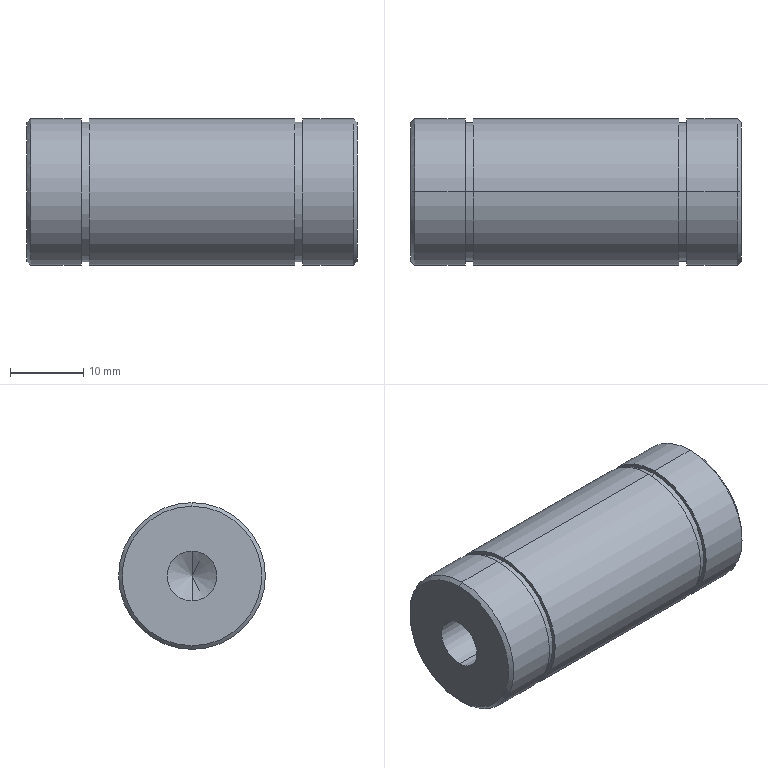Part | SolidWorks | features MirrorPattern 2, Chamfer 1, Extrusion 1, HoleWzd 1, RevCut 1 | 1 solid | 28 faces | box 45 x 20 x 20 mm | volume 12570 mm3 | cylinder 14 | cone 8 | plane 6 | commonest cylinder face diameters 20 x6 6.8 x4 19 x4
STEP:
#1=CARTESIAN_POINT('',(22.,0.,10.));
#2=VERTEX_POINT('',#1);
#3=CARTESIAN_POINT('',(22.,0.,-10.));
#4=VERTEX_POINT('',#3);
#5=CARTESIAN_POINT('',(22.,0.,0.));
#6=DIRECTION('',(-1.,0.,0.));
#7=DIRECTION('',(0.,0.,-1.));
#8=AXIS2_PLACEMENT_3D('',#5,#6,#7);
#9=CIRCLE('',#8,10.);
#10=EDGE_CURVE('',#2,#4,#9,.T.);
#11=ORIENTED_EDGE('',*,*,#10,.T.);
#12=CARTESIAN_POINT('',(15.1,0.,-10.));
#13=VERTEX_POINT('',#12);
#14=CARTESIAN_POINT('',(22.5,0.,-10.));
#15=DIRECTION('',(-1.,0.,0.));
#16=VECTOR('',#15,1000.);
#17=LINE('',#14,#16);
#18=EDGE_CURVE('',#4,#13,#17,.T.);
#19=ORIENTED_EDGE('',*,*,#18,.T.);
#20=CARTESIAN_POINT('',(15.1,0.,10.));
#21=VERTEX_POINT('',#20);
#22=CARTESIAN_POINT('',(15.1,0.,0.));
#23=DIRECTION('',(-1.,0.,0.));
#24=DIRECTION('',(0.,0.,1.));
#25=AXIS2_PLACEMENT_3D('',#22,#23,#24);
#26=CIRCLE('',#25,10.);
#27=EDGE_CURVE('',#21,#13,#26,.T.);
#28=ORIENTED_EDGE('',*,*,#27,.F.);
#29=CARTESIAN_POINT('',(22.5,0.,10.));
#30=DIRECTION('',(-1.,0.,0.));
#31=VECTOR('',#30,1000.);
#32=LINE('',#29,#31);
#33=EDGE_CURVE('',#2,#21,#32,.T.);
#34=ORIENTED_EDGE('',*,*,#33,.F.);
#35=EDGE_LOOP('',(#11,#19,#28,#34));
#36=FACE_OUTER_BOUND('',#35,.T.);
#37=CARTESIAN_POINT('',(22.5,0.,0.));
#38=DIRECTION('',(-1.,0.,0.));
#39=DIRECTION('',(0.,0.,1.));
#40=AXIS2_PLACEMENT_3D('',#37,#38,#39);
#41=CYLINDRICAL_SURFACE('',#40,10.);
#42=ADVANCED_FACE('',(#36),#41,.T.);
#43=CARTESIAN_POINT('',(22.5,0.,-9.5));
#44=VERTEX_POINT('',#43);
#45=CARTESIAN_POINT('',(22.5,0.,9.5));
#46=VERTEX_POINT('',#45);
#47=CARTESIAN_POINT('',(22.5,0.,0.));
#48=DIRECTION('',(1.,0.,0.));
#49=DIRECTION('',(0.,0.,-1.));
#50=AXIS2_PLACEMENT_3D('',#47,#48,#49);
#51=CIRCLE('',#50,9.5);
#52=EDGE_CURVE('',#44,#46,#51,.T.);
#53=ORIENTED_EDGE('',*,*,#52,.F.);
#54=CARTESIAN_POINT('',(22.5,0.,-9.5));
#55=DIRECTION('',(-0.7071,0.,-0.7071));
#56=VECTOR('',#55,1000.);
#57=LINE('',#54,#56);
#58=EDGE_CURVE('',#44,#4,#57,.T.);
#59=ORIENTED_EDGE('',*,*,#58,.T.);
#60=ORIENTED_EDGE('',*,*,#10,.F.);
#61=CARTESIAN_POINT('',(22.5,0.,9.5));
#62=DIRECTION('',(-0.7071,0.,0.7071));
#63=VECTOR('',#62,1000.);
#64=LINE('',#61,#63);
#65=EDGE_CURVE('',#46,#2,#64,.T.);
#66=ORIENTED_EDGE('',*,*,#65,.F.);
#67=EDGE_LOOP('',(#53,#59,#60,#66));
#68=FACE_OUTER_BOUND('',#67,.T.);
#69=CARTESIAN_POINT('',(22.5,0.,0.));
#70=DIRECTION('',(-1.,0.,0.));
#71=DIRECTION('',(0.,0.,1.));
#72=AXIS2_PLACEMENT_3D('',#69,#70,#71);
#73=CONICAL_SURFACE('',#72,9.5,0.7854);
#74=ADVANCED_FACE('',(#68),#73,.T.);
#75=CARTESIAN_POINT('',(2.75,0.,3.4));
#76=VERTEX_POINT('',#75);
#77=CARTESIAN_POINT('',(2.75,0.,-3.4));
#78=VERTEX_POINT('',#77);
#79=CARTESIAN_POINT('',(2.75,0.,0.));
#80=DIRECTION('',(1.,0.,0.));
#81=DIRECTION('',(0.,0.,-1.));
#82=AXIS2_PLACEMENT_3D('',#79,#80,#81);
#83=CIRCLE('',#82,3.4);
#84=EDGE_CURVE('',#76,#78,#83,.T.);
#85=ORIENTED_EDGE('',*,*,#84,.F.);
#86=CARTESIAN_POINT('',(22.5,0.,3.4));
#87=VERTEX_POINT('',#86);
#88=CARTESIAN_POINT('',(22.5,0.,3.4));
#89=DIRECTION('',(1.,0.,0.));
#90=VECTOR('',#89,1000.);
#91=LINE('',#88,#90);
#92=EDGE_CURVE('',#76,#87,#91,.T.);
#93=ORIENTED_EDGE('',*,*,#92,.T.);
#94=CARTESIAN_POINT('',(22.5,0.,-3.4));
#95=VERTEX_POINT('',#94);
#96=CARTESIAN_POINT('',(22.5,0.,0.));
#97=DIRECTION('',(1.,0.,0.));
#98=DIRECTION('',(0.,0.,-1.));
#99=AXIS2_PLACEMENT_3D('',#96,#97,#98);
#100=CIRCLE('',#99,3.4);
#101=EDGE_CURVE('',#87,#95,#100,.T.);
#102=ORIENTED_EDGE('',*,*,#101,.T.);
#103=CARTESIAN_POINT('',(22.5,0.,-3.4));
#104=DIRECTION('',(1.,0.,0.));
#105=VECTOR('',#104,1000.);
#106=LINE('',#103,#105);
#107=EDGE_CURVE('',#78,#95,#106,.T.);
#108=ORIENTED_EDGE('',*,*,#107,.F.);
#109=EDGE_LOOP('',(#85,#93,#102,#108));
#110=FACE_OUTER_BOUND('',#109,.T.);
#111=CARTESIAN_POINT('',(22.5,0.,0.));
#112=DIRECTION('',(1.,0.,0.));
#113=DIRECTION('',(0.,0.,-1.));
#114=AXIS2_PLACEMENT_3D('',#111,#112,#113);
#115=CYLINDRICAL_SURFACE('',#114,3.4);
#116=ADVANCED_FACE('',(#110),#115,.F.);
#117=CARTESIAN_POINT('',(0.7071,0.,0.));
#118=VERTEX_POINT('',#117);
#119=CARTESIAN_POINT('',(2.75,0.,-3.4));
#120=DIRECTION('',(0.515,0.,-0.8572));
#121=VECTOR('',#120,1000.);
#122=LINE('',#119,#121);
#123=EDGE_CURVE('',#118,#78,#122,.T.);
#124=ORIENTED_EDGE('',*,*,#123,.F.);
#125=CARTESIAN_POINT('',(2.75,0.,3.4));
#126=DIRECTION('',(0.515,0.,0.8572));
#127=VECTOR('',#126,1000.);
#128=LINE('',#125,#127);
#129=EDGE_CURVE('',#118,#76,#128,.T.);
#130=ORIENTED_EDGE('',*,*,#129,.T.);
#131=ORIENTED_EDGE('',*,*,#84,.T.);
#132=EDGE_LOOP('',(#124,#130,#131));
#133=FACE_OUTER_BOUND('',#132,.T.);
#134=CARTESIAN_POINT('',(2.75,0.,0.));
#135=DIRECTION('',(1.,0.,0.));
#136=DIRECTION('',(0.,0.,-1.));
#137=AXIS2_PLACEMENT_3D('',#134,#135,#136);
#138=CONICAL_SURFACE('',#137,3.4,1.03);
#139=ADVANCED_FACE('',(#133),#138,.F.);
#140=CARTESIAN_POINT('',(14.,0.,-9.5));
#141=VERTEX_POINT('',#140);
#142=CARTESIAN_POINT('',(14.,0.,9.5));
#143=VERTEX_POINT('',#142);
#144=CARTESIAN_POINT('',(14.,0.,0.));
#145=DIRECTION('',(-1.,0.,0.));
#146=DIRECTION('',(0.,0.,1.));
#147=AXIS2_PLACEMENT_3D('',#144,#145,#146);
#148=CIRCLE('',#147,9.5);
#149=EDGE_CURVE('',#141,#143,#148,.T.);
#150=ORIENTED_EDGE('',*,*,#149,.F.);
#151=CARTESIAN_POINT('',(15.1,0.,-9.5));
#152=VERTEX_POINT('',#151);
#153=CARTESIAN_POINT('',(0.,0.,-9.5));
#154=DIRECTION('',(1.,0.,0.));
#155=VECTOR('',#154,1000.);
#156=LINE('',#153,#155);
#157=EDGE_CURVE('',#141,#152,#156,.T.);
#158=ORIENTED_EDGE('',*,*,#157,.T.);
#159=CARTESIAN_POINT('',(15.1,0.,9.5));
#160=VERTEX_POINT('',#159);
#161=CARTESIAN_POINT('',(15.1,0.,0.));
#162=DIRECTION('',(-1.,0.,0.));
#163=DIRECTION('',(0.,0.,1.));
#164=AXIS2_PLACEMENT_3D('',#161,#162,#163);
#165=CIRCLE('',#164,9.5);
#166=EDGE_CURVE('',#152,#160,#165,.T.);
#167=ORIENTED_EDGE('',*,*,#166,.T.);
#168=CARTESIAN_POINT('',(0.,0.,9.5));
#169=DIRECTION('',(1.,0.,0.));
#170=VECTOR('',#169,1000.);
#171=LINE('',#168,#170);
#172=EDGE_CURVE('',#143,#160,#171,.T.);
#173=ORIENTED_EDGE('',*,*,#172,.F.);
#174=EDGE_LOOP('',(#150,#158,#167,#173));
#175=FACE_OUTER_BOUND('',#174,.T.);
#176=CARTESIAN_POINT('',(0.,0.,0.));
#177=DIRECTION('',(1.,0.,0.));
#178=DIRECTION('',(0.,0.,1.));
#179=AXIS2_PLACEMENT_3D('',#176,#177,#178);
#180=CYLINDRICAL_SURFACE('',#179,9.5);
#181=ADVANCED_FACE('',(#175),#180,.T.);
#182=CARTESIAN_POINT('',(-14.,0.,9.5));
#183=VERTEX_POINT('',#182);
#184=CARTESIAN_POINT('',(-14.,0.,-9.5));
#185=VERTEX_POINT('',#184);
#186=CARTESIAN_POINT('',(-14.,0.,0.));
#187=DIRECTION('',(-1.,0.,0.));
#188=DIRECTION('',(0.,0.,1.));
#189=AXIS2_PLACEMENT_3D('',#186,#187,#188);
#190=CIRCLE('',#189,9.5);
#191=EDGE_CURVE('',#183,#185,#190,.T.);
#192=ORIENTED_EDGE('',*,*,#191,.T.);
#193=CARTESIAN_POINT('',(-15.1,0.,-9.5));
#194=VERTEX_POINT('',#193);
#195=CARTESIAN_POINT('',(0.,0.,-9.5));
#196=DIRECTION('',(-1.,0.,0.));
#197=VECTOR('',#196,1000.);
#198=LINE('',#195,#197);
#199=EDGE_CURVE('',#185,#194,#198,.T.);
#200=ORIENTED_EDGE('',*,*,#199,.T.);
#201=CARTESIAN_POINT('',(-15.1,0.,9.5));
#202=VERTEX_POINT('',#201);
#203=CARTESIAN_POINT('',(-15.1,0.,0.));
#204=DIRECTION('',(-1.,0.,0.));
#205=DIRECTION('',(0.,0.,1.));
#206=AXIS2_PLACEMENT_3D('',#203,#204,#205);
#207=CIRCLE('',#206,9.5);
#208=EDGE_CURVE('',#202,#194,#207,.T.);
#209=ORIENTED_EDGE('',*,*,#208,.F.);
#210=CARTESIAN_POINT('',(0.,0.,9.5));
#211=DIRECTION('',(-1.,0.,0.));
#212=VECTOR('',#211,1000.);
#213=LINE('',#210,#212);
#214=EDGE_CURVE('',#183,#202,#213,.T.);
#215=ORIENTED_EDGE('',*,*,#214,.F.);
#216=EDGE_LOOP('',(#192,#200,#209,#215));
#217=FACE_OUTER_BOUND('',#216,.T.);
#218=CARTESIAN_POINT('',(0.,0.,0.));
#219=DIRECTION('',(-1.,0.,0.));
#220=DIRECTION('',(0.,0.,1.));
#221=AXIS2_PLACEMENT_3D('',#218,#219,#220);
#222=CYLINDRICAL_SURFACE('',#221,9.5);
#223=ADVANCED_FACE('',(#217),#222,.T.);
#224=CARTESIAN_POINT('',(-22.5,0.,9.5));
#225=VERTEX_POINT('',#224);
#226=CARTESIAN_POINT('',(-22.5,0.,-9.5));
#227=VERTEX_POINT('',#226);
#228=CARTESIAN_POINT('',(-22.5,0.,0.));
#229=DIRECTION('',(-1.,0.,0.));
#230=DIRECTION('',(0.,0.,-1.));
#231=AXIS2_PLACEMENT_3D('',#228,#229,#230);
#232=CIRCLE('',#231,9.5);
#233=EDGE_CURVE('',#225,#227,#232,.T.);
#234=ORIENTED_EDGE('',*,*,#233,.F.);
#235=CARTESIAN_POINT('',(-22.,0.,10.));
#236=VERTEX_POINT('',#235);
#237=CARTESIAN_POINT('',(-22.,0.,10.));
#238=DIRECTION('',(0.7071,0.,0.7071));
#239=VECTOR('',#238,1000.);
#240=LINE('',#237,#239);
#241=EDGE_CURVE('',#225,#236,#240,.T.);
#242=ORIENTED_EDGE('',*,*,#241,.T.);
#243=CARTESIAN_POINT('',(-22.,0.,-10.));
#244=VERTEX_POINT('',#243);
#245=CARTESIAN_POINT('',(-22.,0.,0.));
#246=DIRECTION('',(1.,0.,0.));
#247=DIRECTION('',(0.,0.,-1.));
#248=AXIS2_PLACEMENT_3D('',#245,#246,#247);
#249=CIRCLE('',#248,10.);
#250=EDGE_CURVE('',#244,#236,#249,.T.);
#251=ORIENTED_EDGE('',*,*,#250,.F.);
#252=CARTESIAN_POINT('',(-22.,0.,-10.));
#253=DIRECTION('',(0.7071,0.,-0.7071));
#254=VECTOR('',#253,1000.);
#255=LINE('',#252,#254);
#256=EDGE_CURVE('',#227,#244,#255,.T.);
#257=ORIENTED_EDGE('',*,*,#256,.F.);
#258=EDGE_LOOP('',(#234,#242,#251,#257));
#259=FACE_OUTER_BOUND('',#258,.T.);
#260=CARTESIAN_POINT('',(-22.,0.,0.));
#261=DIRECTION('',(1.,0.,0.));
#262=DIRECTION('',(0.,0.,-1.));
#263=AXIS2_PLACEMENT_3D('',#260,#261,#262);
#264=CONICAL_SURFACE('',#263,10.,0.7854);
#265=ADVANCED_FACE('',(#259),#264,.T.);
#266=CARTESIAN_POINT('',(-2.75,0.,-3.4));
#267=VERTEX_POINT('',#266);
#268=CARTESIAN_POINT('',(-2.75,0.,3.4));
#269=VERTEX_POINT('',#268);
#270=CARTESIAN_POINT('',(-2.75,0.,0.));
#271=DIRECTION('',(-1.,0.,0.));
#272=DIRECTION('',(0.,0.,1.));
#273=AXIS2_PLACEMENT_3D('',#270,#271,#272);
#274=CIRCLE('',#273,3.4);
#275=EDGE_CURVE('',#267,#269,#274,.T.);
#276=ORIENTED_EDGE('',*,*,#275,.F.);
#277=CARTESIAN_POINT('',(-22.5,0.,-3.4));
#278=VERTEX_POINT('',#277);
#279=CARTESIAN_POINT('',(-22.5,0.,-3.4));
#280=DIRECTION('',(-1.,0.,0.));
#281=VECTOR('',#280,1000.);
#282=LINE('',#279,#281);
#283=EDGE_CURVE('',#267,#278,#282,.T.);
#284=ORIENTED_EDGE('',*,*,#283,.T.);
#285=CARTESIAN_POINT('',(-22.5,0.,3.4));
#286=VERTEX_POINT('',#285);
#287=CARTESIAN_POINT('',(-22.5,0.,0.));
#288=DIRECTION('',(-1.,0.,0.));
#289=DIRECTION('',(0.,0.,1.));
#290=AXIS2_PLACEMENT_3D('',#287,#288,#289);
#291=CIRCLE('',#290,3.4);
#292=EDGE_CURVE('',#278,#286,#291,.T.);
#293=ORIENTED_EDGE('',*,*,#292,.T.);
#294=CARTESIAN_POINT('',(-22.5,0.,3.4));
#295=DIRECTION('',(-1.,0.,0.));
#296=VECTOR('',#295,1000.);
#297=LINE('',#294,#296);
#298=EDGE_CURVE('',#269,#286,#297,.T.);
#299=ORIENTED_EDGE('',*,*,#298,.F.);
#300=EDGE_LOOP('',(#276,#284,#293,#299));
#301=FACE_OUTER_BOUND('',#300,.T.);
#302=CARTESIAN_POINT('',(-22.5,0.,0.));
#303=DIRECTION('',(-1.,0.,0.));
#304=DIRECTION('',(0.,0.,1.));
#305=AXIS2_PLACEMENT_3D('',#302,#303,#304);
#306=CYLINDRICAL_SURFACE('',#305,3.4);
#307=ADVANCED_FACE('',(#301),#306,.F.);
#308=CARTESIAN_POINT('',(-0.7071,0.,0.));
#309=VERTEX_POINT('',#308);
#310=CARTESIAN_POINT('',(-2.75,0.,3.4));
#311=DIRECTION('',(-0.515,0.,0.8572));
#312=VECTOR('',#311,1000.);
#313=LINE('',#310,#312);
#314=EDGE_CURVE('',#309,#269,#313,.T.);
#315=ORIENTED_EDGE('',*,*,#314,.F.);
#316=CARTESIAN_POINT('',(-2.75,0.,-3.4));
#317=DIRECTION('',(-0.515,0.,-0.8572));
#318=VECTOR('',#317,1000.);
#319=LINE('',#316,#318);
#320=EDGE_CURVE('',#309,#267,#319,.T.);
#321=ORIENTED_EDGE('',*,*,#320,.T.);
#322=ORIENTED_EDGE('',*,*,#275,.T.);
#323=EDGE_LOOP('',(#315,#321,#322));
#324=FACE_OUTER_BOUND('',#323,.T.);
#325=CARTESIAN_POINT('',(-2.75,0.,0.));
#326=DIRECTION('',(-1.,0.,0.));
#327=DIRECTION('',(0.,0.,1.));
#328=AXIS2_PLACEMENT_3D('',#325,#326,#327);
#329=CONICAL_SURFACE('',#328,3.4,1.03);
#330=ADVANCED_FACE('',(#324),#329,.F.);
#331=CARTESIAN_POINT('',(-15.1,0.,10.));
#332=VERTEX_POINT('',#331);
#333=CARTESIAN_POINT('',(-15.1,0.,-10.));
#334=VERTEX_POINT('',#333);
#335=CARTESIAN_POINT('',(-15.1,0.,0.));
#336=DIRECTION('',(-1.,0.,0.));
#337=DIRECTION('',(0.,0.,1.));
#338=AXIS2_PLACEMENT_3D('',#335,#336,#337);
#339=CIRCLE('',#338,10.);
#340=EDGE_CURVE('',#332,#334,#339,.T.);
#341=ORIENTED_EDGE('',*,*,#340,.T.);
#342=CARTESIAN_POINT('',(22.5,0.,-10.));
#343=DIRECTION('',(-1.,0.,0.));
#344=VECTOR('',#343,1000.);
#345=LINE('',#342,#344);
#346=EDGE_CURVE('',#334,#244,#345,.T.);
#347=ORIENTED_EDGE('',*,*,#346,.T.);
#348=ORIENTED_EDGE('',*,*,#250,.T.);
#349=CARTESIAN_POINT('',(22.5,0.,10.));
#350=DIRECTION('',(-1.,0.,0.));
#351=VECTOR('',#350,1000.);
#352=LINE('',#349,#351);
#353=EDGE_CURVE('',#332,#236,#352,.T.);
#354=ORIENTED_EDGE('',*,*,#353,.F.);
#355=EDGE_LOOP('',(#341,#347,#348,#354));
#356=FACE_OUTER_BOUND('',#355,.T.);
#357=CARTESIAN_POINT('',(22.5,0.,0.));
#358=DIRECTION('',(-1.,0.,0.));
#359=DIRECTION('',(0.,0.,1.));
#360=AXIS2_PLACEMENT_3D('',#357,#358,#359);
#361=CYLINDRICAL_SURFACE('',#360,10.);
#362=ADVANCED_FACE('',(#356),#361,.T.);
#363=CARTESIAN_POINT('',(14.,0.,10.));
#364=VERTEX_POINT('',#363);
#365=CARTESIAN_POINT('',(14.,0.,-10.));
#366=VERTEX_POINT('',#365);
#367=CARTESIAN_POINT('',(14.,0.,0.));
#368=DIRECTION('',(-1.,0.,0.));
#369=DIRECTION('',(0.,0.,1.));
#370=AXIS2_PLACEMENT_3D('',#367,#368,#369);
#371=CIRCLE('',#370,10.);
#372=EDGE_CURVE('',#364,#366,#371,.T.);
#373=ORIENTED_EDGE('',*,*,#372,.T.);
#374=CARTESIAN_POINT('',(-14.,0.,-10.));
#375=VERTEX_POINT('',#374);
#376=CARTESIAN_POINT('',(22.5,0.,-10.));
#377=DIRECTION('',(-1.,0.,0.));
#378=VECTOR('',#377,1000.);
#379=LINE('',#376,#378);
#380=EDGE_CURVE('',#366,#375,#379,.T.);
#381=ORIENTED_EDGE('',*,*,#380,.T.);
#382=CARTESIAN_POINT('',(-14.,0.,10.));
#383=VERTEX_POINT('',#382);
#384=CARTESIAN_POINT('',(-14.,0.,0.));
#385=DIRECTION('',(-1.,0.,0.));
#386=DIRECTION('',(0.,0.,1.));
#387=AXIS2_PLACEMENT_3D('',#384,#385,#386);
#388=CIRCLE('',#387,10.);
#389=EDGE_CURVE('',#383,#375,#388,.T.);
#390=ORIENTED_EDGE('',*,*,#389,.F.);
#391=CARTESIAN_POINT('',(22.5,0.,10.));
#392=DIRECTION('',(-1.,0.,0.));
#393=VECTOR('',#392,1000.);
#394=LINE('',#391,#393);
#395=EDGE_CURVE('',#364,#383,#394,.T.);
#396=ORIENTED_EDGE('',*,*,#395,.F.);
#397=EDGE_LOOP('',(#373,#381,#390,#396));
#398=FACE_OUTER_BOUND('',#397,.T.);
#399=CARTESIAN_POINT('',(22.5,0.,0.));
#400=DIRECTION('',(-1.,0.,0.));
#401=DIRECTION('',(0.,0.,1.));
#402=AXIS2_PLACEMENT_3D('',#399,#400,#401);
#403=CYLINDRICAL_SURFACE('',#402,10.);
#404=ADVANCED_FACE('',(#398),#403,.T.);
#405=ORIENTED_EDGE('',*,*,#380,.F.);
#406=CARTESIAN_POINT('',(14.,0.,0.));
#407=DIRECTION('',(-1.,0.,0.));
#408=DIRECTION('',(0.,0.,1.));
#409=AXIS2_PLACEMENT_3D('',#406,#407,#408);
#410=CIRCLE('',#409,10.);
#411=EDGE_CURVE('',#366,#364,#410,.T.);
#412=ORIENTED_EDGE('',*,*,#411,.T.);
#413=ORIENTED_EDGE('',*,*,#395,.T.);
#414=CARTESIAN_POINT('',(-14.,0.,0.));
#415=DIRECTION('',(-1.,0.,0.));
#416=DIRECTION('',(0.,0.,1.));
#417=AXIS2_PLACEMENT_3D('',#414,#415,#416);
#418=CIRCLE('',#417,10.);
#419=EDGE_CURVE('',#375,#383,#418,.T.);
#420=ORIENTED_EDGE('',*,*,#419,.F.);
#421=EDGE_LOOP('',(#405,#412,#413,#420));
#422=FACE_OUTER_BOUND('',#421,.T.);
#423=CARTESIAN_POINT('',(22.5,0.,0.));
#424=DIRECTION('',(-1.,0.,0.));
#425=DIRECTION('',(0.,0.,1.));
#426=AXIS2_PLACEMENT_3D('',#423,#424,#425);
#427=CYLINDRICAL_SURFACE('',#426,10.);
#428=ADVANCED_FACE('',(#422),#427,.T.);
#429=ORIENTED_EDGE('',*,*,#346,.F.);
#430=CARTESIAN_POINT('',(-15.1,0.,0.));
#431=DIRECTION('',(-1.,0.,0.));
#432=DIRECTION('',(0.,0.,1.));
#433=AXIS2_PLACEMENT_3D('',#430,#431,#432);
#434=CIRCLE('',#433,10.);
#435=EDGE_CURVE('',#334,#332,#434,.T.);
#436=ORIENTED_EDGE('',*,*,#435,.T.);
#437=ORIENTED_EDGE('',*,*,#353,.T.);
#438=CARTESIAN_POINT('',(-22.,0.,0.));
#439=DIRECTION('',(1.,0.,0.));
#440=DIRECTION('',(0.,0.,-1.));
#441=AXIS2_PLACEMENT_3D('',#438,#439,#440);
#442=CIRCLE('',#441,10.);
#443=EDGE_CURVE('',#236,#244,#442,.T.);
#444=ORIENTED_EDGE('',*,*,#443,.T.);
#445=EDGE_LOOP('',(#429,#436,#437,#444));
#446=FACE_OUTER_BOUND('',#445,.T.);
#447=CARTESIAN_POINT('',(22.5,0.,0.));
#448=DIRECTION('',(-1.,0.,0.));
#449=DIRECTION('',(0.,0.,1.));
#450=AXIS2_PLACEMENT_3D('',#447,#448,#449);
#451=CYLINDRICAL_SURFACE('',#450,10.);
#452=ADVANCED_FACE('',(#446),#451,.T.);
#453=CARTESIAN_POINT('',(-22.5,0.,0.));
#454=DIRECTION('',(-1.,0.,0.));
#455=DIRECTION('',(0.,0.,-1.));
#456=AXIS2_PLACEMENT_3D('',#453,#454,#455);
#457=CIRCLE('',#456,9.5);
#458=EDGE_CURVE('',#227,#225,#457,.T.);
#459=ORIENTED_EDGE('',*,*,#458,.T.);
#460=ORIENTED_EDGE('',*,*,#233,.T.);
#461=EDGE_LOOP('',(#459,#460));
#462=FACE_OUTER_BOUND('',#461,.T.);
#463=CARTESIAN_POINT('',(-22.5,0.,0.));
#464=DIRECTION('',(-1.,0.,0.));
#465=DIRECTION('',(0.,0.,1.));
#466=AXIS2_PLACEMENT_3D('',#463,#464,#465);
#467=CIRCLE('',#466,3.4);
#468=EDGE_CURVE('',#286,#278,#467,.T.);
#469=ORIENTED_EDGE('',*,*,#468,.F.);
#470=ORIENTED_EDGE('',*,*,#292,.F.);
#471=EDGE_LOOP('',(#469,#470));
#472=FACE_BOUND('',#471,.T.);
#473=CARTESIAN_POINT('',(-22.5,0.,0.));
#474=DIRECTION('',(1.,0.,0.));
#475=DIRECTION('',(0.,0.,-1.));
#476=AXIS2_PLACEMENT_3D('',#473,#474,#475);
#477=PLANE('',#476);
#478=ADVANCED_FACE('',(#462,#472),#477,.F.);
#479=ORIENTED_EDGE('',*,*,#320,.F.);
#480=ORIENTED_EDGE('',*,*,#314,.T.);
#481=CARTESIAN_POINT('',(-2.75,0.,0.));
#482=DIRECTION('',(-1.,0.,0.));
#483=DIRECTION('',(0.,0.,1.));
#484=AXIS2_PLACEMENT_3D('',#481,#482,#483);
#485=CIRCLE('',#484,3.4);
#486=EDGE_CURVE('',#269,#267,#485,.T.);
#487=ORIENTED_EDGE('',*,*,#486,.T.);
#488=EDGE_LOOP('',(#479,#480,#487));
#489=FACE_OUTER_BOUND('',#488,.T.);
#490=CARTESIAN_POINT('',(-2.75,0.,0.));
#491=DIRECTION('',(-1.,0.,0.));
#492=DIRECTION('',(0.,0.,1.));
#493=AXIS2_PLACEMENT_3D('',#490,#491,#492);
#494=CONICAL_SURFACE('',#493,3.4,1.03);
#495=ADVANCED_FACE('',(#489),#494,.F.);
#496=ORIENTED_EDGE('',*,*,#283,.F.);
#497=ORIENTED_EDGE('',*,*,#486,.F.);
#498=ORIENTED_EDGE('',*,*,#298,.T.);
#499=ORIENTED_EDGE('',*,*,#468,.T.);
#500=EDGE_LOOP('',(#496,#497,#498,#499));
#501=FACE_OUTER_BOUND('',#500,.T.);
#502=CARTESIAN_POINT('',(-22.5,0.,0.));
#503=DIRECTION('',(-1.,0.,0.));
#504=DIRECTION('',(0.,0.,1.));
#505=AXIS2_PLACEMENT_3D('',#502,#503,#504);
#506=CYLINDRICAL_SURFACE('',#505,3.4);
#507=ADVANCED_FACE('',(#501),#506,.F.);
#508=ORIENTED_EDGE('',*,*,#241,.F.);
#509=ORIENTED_EDGE('',*,*,#458,.F.);
#510=ORIENTED_EDGE('',*,*,#256,.T.);
#511=ORIENTED_EDGE('',*,*,#443,.F.);
#512=EDGE_LOOP('',(#508,#509,#510,#511));
#513=FACE_OUTER_BOUND('',#512,.T.);
#514=CARTESIAN_POINT('',(-22.,0.,0.));
#515=DIRECTION('',(1.,0.,0.));
#516=DIRECTION('',(0.,0.,-1.));
#517=AXIS2_PLACEMENT_3D('',#514,#515,#516);
#518=CONICAL_SURFACE('',#517,10.,0.7854);
#519=ADVANCED_FACE('',(#513),#518,.T.);
#520=ORIENTED_EDGE('',*,*,#208,.T.);
#521=CARTESIAN_POINT('',(-15.1,0.,0.));
#522=DIRECTION('',(-1.,0.,0.));
#523=DIRECTION('',(0.,0.,1.));
#524=AXIS2_PLACEMENT_3D('',#521,#522,#523);
#525=CIRCLE('',#524,9.5);
#526=EDGE_CURVE('',#194,#202,#525,.T.);
#527=ORIENTED_EDGE('',*,*,#526,.T.);
#528=EDGE_LOOP('',(#520,#527));
#529=FACE_BOUND('',#528,.T.);
#530=ORIENTED_EDGE('',*,*,#340,.F.);
#531=ORIENTED_EDGE('',*,*,#435,.F.);
#532=EDGE_LOOP('',(#530,#531));
#533=FACE_OUTER_BOUND('',#532,.T.);
#534=CARTESIAN_POINT('',(-15.1,10.,0.));
#535=DIRECTION('',(1.,0.,0.));
#536=DIRECTION('',(0.,0.,-1.));
#537=AXIS2_PLACEMENT_3D('',#534,#535,#536);
#538=PLANE('',#537);
#539=ADVANCED_FACE('',(#529,#533),#538,.T.);
#540=ORIENTED_EDGE('',*,*,#199,.F.);
#541=CARTESIAN_POINT('',(-14.,0.,0.));
#542=DIRECTION('',(-1.,0.,0.));
#543=DIRECTION('',(0.,0.,1.));
#544=AXIS2_PLACEMENT_3D('',#541,#542,#543);
#545=CIRCLE('',#544,9.5);
#546=EDGE_CURVE('',#185,#183,#545,.T.);
#547=ORIENTED_EDGE('',*,*,#546,.T.);
#548=ORIENTED_EDGE('',*,*,#214,.T.);
#549=ORIENTED_EDGE('',*,*,#526,.F.);
#550=EDGE_LOOP('',(#540,#547,#548,#549));
#551=FACE_OUTER_BOUND('',#550,.T.);
#552=CARTESIAN_POINT('',(0.,0.,0.));
#553=DIRECTION('',(-1.,0.,0.));
#554=DIRECTION('',(0.,0.,1.));
#555=AXIS2_PLACEMENT_3D('',#552,#553,#554);
#556=CYLINDRICAL_SURFACE('',#555,9.5);
#557=ADVANCED_FACE('',(#551),#556,.T.);
#558=ORIENTED_EDGE('',*,*,#389,.T.);
#559=ORIENTED_EDGE('',*,*,#419,.T.);
#560=EDGE_LOOP('',(#558,#559));
#561=FACE_OUTER_BOUND('',#560,.T.);
#562=ORIENTED_EDGE('',*,*,#191,.F.);
#563=ORIENTED_EDGE('',*,*,#546,.F.);
#564=EDGE_LOOP('',(#562,#563));
#565=FACE_BOUND('',#564,.T.);
#566=CARTESIAN_POINT('',(-14.,10.,0.));
#567=DIRECTION('',(-1.,0.,0.));
#568=DIRECTION('',(0.,0.,1.));
#569=AXIS2_PLACEMENT_3D('',#566,#567,#568);
#570=PLANE('',#569);
#571=ADVANCED_FACE('',(#561,#565),#570,.T.);
#572=CARTESIAN_POINT('',(15.1,0.,0.));
#573=DIRECTION('',(-1.,0.,0.));
#574=DIRECTION('',(0.,0.,1.));
#575=AXIS2_PLACEMENT_3D('',#572,#573,#574);
#576=CIRCLE('',#575,9.5);
#577=EDGE_CURVE('',#160,#152,#576,.T.);
#578=ORIENTED_EDGE('',*,*,#577,.F.);
#579=ORIENTED_EDGE('',*,*,#166,.F.);
#580=EDGE_LOOP('',(#578,#579));
#581=FACE_BOUND('',#580,.T.);
#582=ORIENTED_EDGE('',*,*,#27,.T.);
#583=CARTESIAN_POINT('',(15.1,0.,0.));
#584=DIRECTION('',(-1.,0.,0.));
#585=DIRECTION('',(0.,0.,1.));
#586=AXIS2_PLACEMENT_3D('',#583,#584,#585);
#587=CIRCLE('',#586,10.);
#588=EDGE_CURVE('',#13,#21,#587,.T.);
#589=ORIENTED_EDGE('',*,*,#588,.T.);
#590=EDGE_LOOP('',(#582,#589));
#591=FACE_OUTER_BOUND('',#590,.T.);
#592=CARTESIAN_POINT('',(15.1,10.,0.));
#593=DIRECTION('',(-1.,0.,0.));
#594=DIRECTION('',(0.,0.,-1.));
#595=AXIS2_PLACEMENT_3D('',#592,#593,#594);
#596=PLANE('',#595);
#597=ADVANCED_FACE('',(#581,#591),#596,.T.);
#598=ORIENTED_EDGE('',*,*,#157,.F.);
#599=CARTESIAN_POINT('',(14.,0.,0.));
#600=DIRECTION('',(-1.,0.,0.));
#601=DIRECTION('',(0.,0.,1.));
#602=AXIS2_PLACEMENT_3D('',#599,#600,#601);
#603=CIRCLE('',#602,9.5);
#604=EDGE_CURVE('',#143,#141,#603,.T.);
#605=ORIENTED_EDGE('',*,*,#604,.F.);
#606=ORIENTED_EDGE('',*,*,#172,.T.);
#607=ORIENTED_EDGE('',*,*,#577,.T.);
#608=EDGE_LOOP('',(#598,#605,#606,#607));
#609=FACE_OUTER_BOUND('',#608,.T.);
#610=CARTESIAN_POINT('',(0.,0.,0.));
#611=DIRECTION('',(1.,0.,0.));
#612=DIRECTION('',(0.,0.,1.));
#613=AXIS2_PLACEMENT_3D('',#610,#611,#612);
#614=CYLINDRICAL_SURFACE('',#613,9.5);
#615=ADVANCED_FACE('',(#609),#614,.T.);
#616=ORIENTED_EDGE('',*,*,#372,.F.);
#617=ORIENTED_EDGE('',*,*,#411,.F.);
#618=EDGE_LOOP('',(#616,#617));
#619=FACE_OUTER_BOUND('',#618,.T.);
#620=ORIENTED_EDGE('',*,*,#604,.T.);
#621=ORIENTED_EDGE('',*,*,#149,.T.);
#622=EDGE_LOOP('',(#620,#621));
#623=FACE_BOUND('',#622,.T.);
#624=CARTESIAN_POINT('',(14.,10.,0.));
#625=DIRECTION('',(1.,0.,0.));
#626=DIRECTION('',(0.,0.,1.));
#627=AXIS2_PLACEMENT_3D('',#624,#625,#626);
#628=PLANE('',#627);
#629=ADVANCED_FACE('',(#619,#623),#628,.T.);
#630=ORIENTED_EDGE('',*,*,#129,.F.);
#631=ORIENTED_EDGE('',*,*,#123,.T.);
#632=CARTESIAN_POINT('',(2.75,0.,0.));
#633=DIRECTION('',(1.,0.,0.));
#634=DIRECTION('',(0.,0.,-1.));
#635=AXIS2_PLACEMENT_3D('',#632,#633,#634);
#636=CIRCLE('',#635,3.4);
#637=EDGE_CURVE('',#78,#76,#636,.T.);
#638=ORIENTED_EDGE('',*,*,#637,.T.);
#639=EDGE_LOOP('',(#630,#631,#638));
#640=FACE_OUTER_BOUND('',#639,.T.);
#641=CARTESIAN_POINT('',(2.75,0.,0.));
#642=DIRECTION('',(1.,0.,0.));
#643=DIRECTION('',(0.,0.,-1.));
#644=AXIS2_PLACEMENT_3D('',#641,#642,#643);
#645=CONICAL_SURFACE('',#644,3.4,1.03);
#646=ADVANCED_FACE('',(#640),#645,.F.);
#647=ORIENTED_EDGE('',*,*,#92,.F.);
#648=ORIENTED_EDGE('',*,*,#637,.F.);
#649=ORIENTED_EDGE('',*,*,#107,.T.);
#650=CARTESIAN_POINT('',(22.5,0.,0.));
#651=DIRECTION('',(1.,0.,0.));
#652=DIRECTION('',(0.,0.,-1.));
#653=AXIS2_PLACEMENT_3D('',#650,#651,#652);
#654=CIRCLE('',#653,3.4);
#655=EDGE_CURVE('',#95,#87,#654,.T.);
#656=ORIENTED_EDGE('',*,*,#655,.T.);
#657=EDGE_LOOP('',(#647,#648,#649,#656));
#658=FACE_OUTER_BOUND('',#657,.T.);
#659=CARTESIAN_POINT('',(22.5,0.,0.));
#660=DIRECTION('',(1.,0.,0.));
#661=DIRECTION('',(0.,0.,-1.));
#662=AXIS2_PLACEMENT_3D('',#659,#660,#661);
#663=CYLINDRICAL_SURFACE('',#662,3.4);
#664=ADVANCED_FACE('',(#658),#663,.F.);
#665=CARTESIAN_POINT('',(22.5,0.,0.));
#666=DIRECTION('',(1.,0.,0.));
#667=DIRECTION('',(0.,0.,-1.));
#668=AXIS2_PLACEMENT_3D('',#665,#666,#667);
#669=CIRCLE('',#668,9.5);
#670=EDGE_CURVE('',#46,#44,#669,.T.);
#671=ORIENTED_EDGE('',*,*,#670,.T.);
#672=ORIENTED_EDGE('',*,*,#52,.T.);
#673=EDGE_LOOP('',(#671,#672));
#674=FACE_OUTER_BOUND('',#673,.T.);
#675=ORIENTED_EDGE('',*,*,#655,.F.);
#676=ORIENTED_EDGE('',*,*,#101,.F.);
#677=EDGE_LOOP('',(#675,#676));
#678=FACE_BOUND('',#677,.T.);
#679=CARTESIAN_POINT('',(22.5,0.,0.));
#680=DIRECTION('',(1.,0.,0.));
#681=DIRECTION('',(0.,0.,-1.));
#682=AXIS2_PLACEMENT_3D('',#679,#680,#681);
#683=PLANE('',#682);
#684=ADVANCED_FACE('',(#674,#678),#683,.T.);
#685=ORIENTED_EDGE('',*,*,#58,.F.);
#686=ORIENTED_EDGE('',*,*,#670,.F.);
#687=ORIENTED_EDGE('',*,*,#65,.T.);
#688=CARTESIAN_POINT('',(22.,0.,0.));
#689=DIRECTION('',(-1.,0.,0.));
#690=DIRECTION('',(0.,0.,-1.));
#691=AXIS2_PLACEMENT_3D('',#688,#689,#690);
#692=CIRCLE('',#691,10.);
#693=EDGE_CURVE('',#4,#2,#692,.T.);
#694=ORIENTED_EDGE('',*,*,#693,.F.);
#695=EDGE_LOOP('',(#685,#686,#687,#694));
#696=FACE_OUTER_BOUND('',#695,.T.);
#697=CARTESIAN_POINT('',(22.5,0.,0.));
#698=DIRECTION('',(-1.,0.,0.));
#699=DIRECTION('',(0.,0.,1.));
#700=AXIS2_PLACEMENT_3D('',#697,#698,#699);
#701=CONICAL_SURFACE('',#700,9.5,0.7854);
#702=ADVANCED_FACE('',(#696),#701,.T.);
#703=ORIENTED_EDGE('',*,*,#18,.F.);
#704=ORIENTED_EDGE('',*,*,#693,.T.);
#705=ORIENTED_EDGE('',*,*,#33,.T.);
#706=ORIENTED_EDGE('',*,*,#588,.F.);
#707=EDGE_LOOP('',(#703,#704,#705,#706));
#708=FACE_OUTER_BOUND('',#707,.T.);
#709=CARTESIAN_POINT('',(22.5,0.,0.));
#710=DIRECTION('',(-1.,0.,0.));
#711=DIRECTION('',(0.,0.,1.));
#712=AXIS2_PLACEMENT_3D('',#709,#710,#711);
#713=CYLINDRICAL_SURFACE('',#712,10.);
#714=ADVANCED_FACE('',(#708),#713,.T.);
#715=CLOSED_SHELL('',(#42,#74,#116,#139,#181,#223,#265,#307,#330,#362,#404,#428,#452,#478,#495,#507,#519,#539,#557,#571,#597,#615,#629,#646,#664,#684,#702,#714));
#716=MANIFOLD_SOLID_BREP('',#715);
#717=CARTESIAN_POINT('',(0.,0.,0.));
#718=DIRECTION('',(0.,0.,1.));
#719=DIRECTION('',(1.,0.,0.));
#720=AXIS2_PLACEMENT_3D('',#717,#718,#719);
#721=(LENGTH_UNIT()NAMED_UNIT(*)SI_UNIT(.MILLI.,.METRE.));
#722=UNCERTAINTY_MEASURE_WITH_UNIT(LENGTH_MEASURE(0.00001),#721,'','');
#723=(NAMED_UNIT(*)PLANE_ANGLE_UNIT()SI_UNIT($,.RADIAN.));
#724=(NAMED_UNIT(*)SI_UNIT($,.STERADIAN.)SOLID_ANGLE_UNIT());
#725=(GEOMETRIC_REPRESENTATION_CONTEXT(3)GLOBAL_UNCERTAINTY_ASSIGNED_CONTEXT((#722))GLOBAL_UNIT_ASSIGNED_CONTEXT((#721,#723,#724))REPRESENTATION_CONTEXT('',''));
#726=ADVANCED_BREP_SHAPE_REPRESENTATION('',(#716,#720),#725);